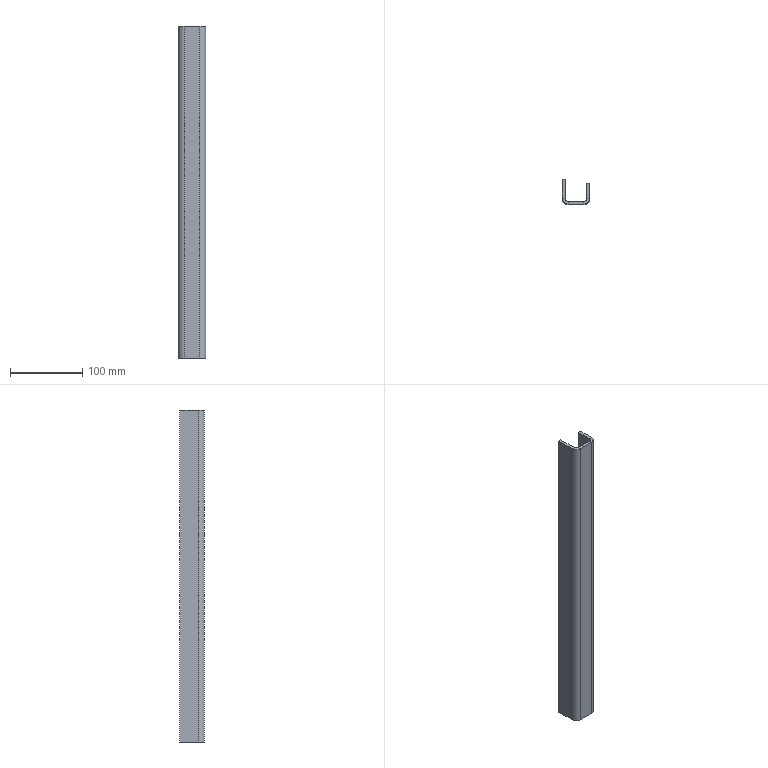Part | STEP file | 07-Reinforcing bent plate 2 | 1 solid | 22 faces | box 38 x 34 x 459 mm | volume 161170 mm3 | plane 18 | cylinder 4 | commonest cylinder face diameters 8 x2 16 x2
STEP:
#1=CARTESIAN_POINT('',(0.,0.,0.));
#2=DIRECTION('',(0.,0.,1.));
#3=DIRECTION('',(1.,0.,0.));
#4=AXIS2_PLACEMENT_3D('',#1,#2,#3);
#5=CARTESIAN_POINT('',(0.,-26.,459.));
#6=VERTEX_POINT('',#5);
#7=CARTESIAN_POINT('',(4.,-26.,459.));
#8=VERTEX_POINT('',#7);
#9=CARTESIAN_POINT('',(0.,-26.,459.));
#10=DIRECTION('',(1.,0.,0.));
#11=VECTOR('',#10,1.);
#12=LINE('',#9,#11);
#13=CARTESIAN_POINT('',(0.,-26.,459.));
#14=DIRECTION('',(0.,0.,1.));
#15=DIRECTION('',(1.,0.,0.));
#16=AXIS2_PLACEMENT_3D('',#13,#14,#15);
#17=PLANE('',#16);
#18=CARTESIAN_POINT('',(0.,0.));
#19=DIRECTION('',(1.,0.));
#20=VECTOR('',#19,1.);
#21=LINE('',#18,#20);
#22=(GEOMETRIC_REPRESENTATION_CONTEXT(2)PARAMETRIC_REPRESENTATION_CONTEXT()REPRESENTATION_CONTEXT('',''));
#23=DEFINITIONAL_REPRESENTATION('',(#21),#22);
#24=PCURVE('',#17,#23);
#25=CARTESIAN_POINT('',(8.,-30.,459.));
#26=DIRECTION('',(0.,0.,1.));
#27=DIRECTION('',(1.,0.,0.));
#28=AXIS2_PLACEMENT_3D('',#25,#26,#27);
#29=PLANE('',#28);
#30=CARTESIAN_POINT('',(-8.,4.));
#31=DIRECTION('',(1.,0.));
#32=VECTOR('',#31,1.);
#33=LINE('',#30,#32);
#34=(GEOMETRIC_REPRESENTATION_CONTEXT(2)PARAMETRIC_REPRESENTATION_CONTEXT()REPRESENTATION_CONTEXT('',''));
#35=DEFINITIONAL_REPRESENTATION('',(#33),#34);
#36=PCURVE('',#29,#35);
#37=SURFACE_CURVE('',#12,(#24,#36),.PCURVE_S1.);
#38=EDGE_CURVE('',#6,#8,#37,.T.);
#39=ORIENTED_EDGE('',*,*,#38,.F.);
#40=CARTESIAN_POINT('',(8.,-34.,459.));
#41=VERTEX_POINT('',#40);
#42=CARTESIAN_POINT('',(8.,-26.,459.));
#43=DIRECTION('',(0.,0.,1.));
#44=DIRECTION('',(-1.,0.,0.));
#45=AXIS2_PLACEMENT_3D('',#42,#43,#44);
#46=CIRCLE('',#45,8.);
#47=CARTESIAN_POINT('',(8.,0.));
#48=DIRECTION('',(-1.,0.));
#49=AXIS2_PLACEMENT_2D('',#47,#48);
#50=CIRCLE('',#49,8.);
#51=(GEOMETRIC_REPRESENTATION_CONTEXT(2)PARAMETRIC_REPRESENTATION_CONTEXT()REPRESENTATION_CONTEXT('',''));
#52=DEFINITIONAL_REPRESENTATION('',(#50),#51);
#53=PCURVE('',#17,#52);
#54=CARTESIAN_POINT('',(8.,-26.,459.));
#55=DIRECTION('',(0.,0.,-1.));
#56=DIRECTION('',(-1.,0.,0.));
#57=AXIS2_PLACEMENT_3D('',#54,#55,#56);
#58=CYLINDRICAL_SURFACE('',#57,8.);
#59=CARTESIAN_POINT('',(6.283,0.));
#60=DIRECTION('',(-1.,0.));
#61=VECTOR('',#60,1.);
#62=LINE('',#59,#61);
#63=(GEOMETRIC_REPRESENTATION_CONTEXT(2)PARAMETRIC_REPRESENTATION_CONTEXT()REPRESENTATION_CONTEXT('',''));
#64=DEFINITIONAL_REPRESENTATION('',(#62),#63);
#65=PCURVE('',#58,#64);
#66=SURFACE_CURVE('',#46,(#53,#65),.PCURVE_S1.);
#67=EDGE_CURVE('',#6,#41,#66,.T.);
#68=ORIENTED_EDGE('',*,*,#67,.T.);
#69=CARTESIAN_POINT('',(8.,-30.,459.));
#70=VERTEX_POINT('',#69);
#71=CARTESIAN_POINT('',(8.,-30.,459.));
#72=DIRECTION('',(0.,-1.,0.));
#73=VECTOR('',#72,1.);
#74=LINE('',#71,#73);
#75=CARTESIAN_POINT('',(8.,-4.));
#76=DIRECTION('',(0.,-1.));
#77=VECTOR('',#76,1.);
#78=LINE('',#75,#77);
#79=(GEOMETRIC_REPRESENTATION_CONTEXT(2)PARAMETRIC_REPRESENTATION_CONTEXT()REPRESENTATION_CONTEXT('',''));
#80=DEFINITIONAL_REPRESENTATION('',(#78),#79);
#81=PCURVE('',#17,#80);
#82=CARTESIAN_POINT('',(34.,-26.,459.));
#83=DIRECTION('',(0.,0.,1.));
#84=DIRECTION('',(1.,0.,0.));
#85=AXIS2_PLACEMENT_3D('',#82,#83,#84);
#86=PLANE('',#85);
#87=CARTESIAN_POINT('',(-26.,-4.));
#88=DIRECTION('',(0.,-1.));
#89=VECTOR('',#88,1.);
#90=LINE('',#87,#89);
#91=(GEOMETRIC_REPRESENTATION_CONTEXT(2)PARAMETRIC_REPRESENTATION_CONTEXT()REPRESENTATION_CONTEXT('',''));
#92=DEFINITIONAL_REPRESENTATION('',(#90),#91);
#93=PCURVE('',#86,#92);
#94=SURFACE_CURVE('',#74,(#81,#93),.PCURVE_S1.);
#95=EDGE_CURVE('',#70,#41,#94,.T.);
#96=ORIENTED_EDGE('',*,*,#95,.F.);
#97=CARTESIAN_POINT('',(8.,-26.,459.));
#98=DIRECTION('',(0.,0.,1.));
#99=DIRECTION('',(1.,0.,0.));
#100=AXIS2_PLACEMENT_3D('',#97,#98,#99);
#101=CIRCLE('',#100,4.);
#102=CARTESIAN_POINT('',(8.,0.));
#103=DIRECTION('',(1.,0.));
#104=AXIS2_PLACEMENT_2D('',#102,#103);
#105=CIRCLE('',#104,4.);
#106=(GEOMETRIC_REPRESENTATION_CONTEXT(2)PARAMETRIC_REPRESENTATION_CONTEXT()REPRESENTATION_CONTEXT('',''));
#107=DEFINITIONAL_REPRESENTATION('',(#105),#106);
#108=PCURVE('',#17,#107);
#109=CARTESIAN_POINT('',(8.,-26.,459.));
#110=DIRECTION('',(0.,0.,-1.));
#111=DIRECTION('',(-1.,0.,0.));
#112=AXIS2_PLACEMENT_3D('',#109,#110,#111);
#113=CYLINDRICAL_SURFACE('',#112,4.);
#114=CARTESIAN_POINT('',(9.425,0.));
#115=DIRECTION('',(-1.,0.));
#116=VECTOR('',#115,1.);
#117=LINE('',#114,#116);
#118=(GEOMETRIC_REPRESENTATION_CONTEXT(2)PARAMETRIC_REPRESENTATION_CONTEXT()REPRESENTATION_CONTEXT('',''));
#119=DEFINITIONAL_REPRESENTATION('',(#117),#118);
#120=PCURVE('',#113,#119);
#121=SURFACE_CURVE('',#101,(#108,#120),.PCURVE_S1.);
#122=EDGE_CURVE('',#8,#70,#121,.T.);
#123=ORIENTED_EDGE('',*,*,#122,.F.);
#124=EDGE_LOOP('',(#39,#68,#96,#123));
#125=FACE_BOUND('',#124,.T.);
#126=ADVANCED_FACE('',(#125),#17,.T.);
#127=CARTESIAN_POINT('',(0.,0.,459.));
#128=VERTEX_POINT('',#127);
#129=CARTESIAN_POINT('',(0.,0.,459.));
#130=DIRECTION('',(0.,-1.,0.));
#131=VECTOR('',#130,1.);
#132=LINE('',#129,#131);
#133=CARTESIAN_POINT('',(-8.,30.));
#134=DIRECTION('',(0.,-1.));
#135=VECTOR('',#134,1.);
#136=LINE('',#133,#135);
#137=(GEOMETRIC_REPRESENTATION_CONTEXT(2)PARAMETRIC_REPRESENTATION_CONTEXT()REPRESENTATION_CONTEXT('',''));
#138=DEFINITIONAL_REPRESENTATION('',(#136),#137);
#139=PCURVE('',#29,#138);
#140=CARTESIAN_POINT('',(0.,0.,459.));
#141=DIRECTION('',(1.,0.,0.));
#142=DIRECTION('',(0.,1.,0.));
#143=AXIS2_PLACEMENT_3D('',#140,#141,#142);
#144=PLANE('',#143);
#145=CARTESIAN_POINT('',(0.,0.));
#146=DIRECTION('',(-1.,0.));
#147=VECTOR('',#146,1.);
#148=LINE('',#145,#147);
#149=(GEOMETRIC_REPRESENTATION_CONTEXT(2)PARAMETRIC_REPRESENTATION_CONTEXT()REPRESENTATION_CONTEXT('',''));
#150=DEFINITIONAL_REPRESENTATION('',(#148),#149);
#151=PCURVE('',#144,#150);
#152=SURFACE_CURVE('',#132,(#139,#151),.PCURVE_S1.);
#153=EDGE_CURVE('',#128,#6,#152,.T.);
#154=ORIENTED_EDGE('',*,*,#153,.T.);
#155=ORIENTED_EDGE('',*,*,#38,.T.);
#156=CARTESIAN_POINT('',(4.,0.,459.));
#157=VERTEX_POINT('',#156);
#158=CARTESIAN_POINT('',(4.,0.,459.));
#159=DIRECTION('',(0.,-1.,0.));
#160=VECTOR('',#159,1.);
#161=LINE('',#158,#160);
#162=CARTESIAN_POINT('',(-4.,30.));
#163=DIRECTION('',(0.,-1.));
#164=VECTOR('',#163,1.);
#165=LINE('',#162,#164);
#166=(GEOMETRIC_REPRESENTATION_CONTEXT(2)PARAMETRIC_REPRESENTATION_CONTEXT()REPRESENTATION_CONTEXT('',''));
#167=DEFINITIONAL_REPRESENTATION('',(#165),#166);
#168=PCURVE('',#29,#167);
#169=CARTESIAN_POINT('',(4.,0.,459.));
#170=DIRECTION('',(1.,0.,0.));
#171=DIRECTION('',(0.,1.,0.));
#172=AXIS2_PLACEMENT_3D('',#169,#170,#171);
#173=PLANE('',#172);
#174=CARTESIAN_POINT('',(0.,0.));
#175=DIRECTION('',(-1.,0.));
#176=VECTOR('',#175,1.);
#177=LINE('',#174,#176);
#178=(GEOMETRIC_REPRESENTATION_CONTEXT(2)PARAMETRIC_REPRESENTATION_CONTEXT()REPRESENTATION_CONTEXT('',''));
#179=DEFINITIONAL_REPRESENTATION('',(#177),#178);
#180=PCURVE('',#173,#179);
#181=SURFACE_CURVE('',#161,(#168,#180),.PCURVE_S1.);
#182=EDGE_CURVE('',#157,#8,#181,.T.);
#183=ORIENTED_EDGE('',*,*,#182,.F.);
#184=CARTESIAN_POINT('',(0.,0.,459.));
#185=DIRECTION('',(1.,0.,0.));
#186=VECTOR('',#185,1.);
#187=LINE('',#184,#186);
#188=CARTESIAN_POINT('',(-8.,30.));
#189=DIRECTION('',(1.,0.));
#190=VECTOR('',#189,1.);
#191=LINE('',#188,#190);
#192=(GEOMETRIC_REPRESENTATION_CONTEXT(2)PARAMETRIC_REPRESENTATION_CONTEXT()REPRESENTATION_CONTEXT('',''));
#193=DEFINITIONAL_REPRESENTATION('',(#191),#192);
#194=PCURVE('',#29,#193);
#195=CARTESIAN_POINT('',(0.,0.,459.));
#196=DIRECTION('',(0.,1.,0.));
#197=DIRECTION('',(-1.,0.,0.));
#198=AXIS2_PLACEMENT_3D('',#195,#196,#197);
#199=PLANE('',#198);
#200=CARTESIAN_POINT('',(0.,0.));
#201=DIRECTION('',(-1.,0.));
#202=VECTOR('',#201,1.);
#203=LINE('',#200,#202);
#204=(GEOMETRIC_REPRESENTATION_CONTEXT(2)PARAMETRIC_REPRESENTATION_CONTEXT()REPRESENTATION_CONTEXT('',''));
#205=DEFINITIONAL_REPRESENTATION('',(#203),#204);
#206=PCURVE('',#199,#205);
#207=SURFACE_CURVE('',#187,(#194,#206),.PCURVE_S1.);
#208=EDGE_CURVE('',#128,#157,#207,.T.);
#209=ORIENTED_EDGE('',*,*,#208,.F.);
#210=EDGE_LOOP('',(#154,#155,#183,#209));
#211=FACE_BOUND('',#210,.T.);
#212=ADVANCED_FACE('',(#211),#29,.T.);
#213=CARTESIAN_POINT('',(8.,-34.,0.));
#214=VERTEX_POINT('',#213);
#215=CARTESIAN_POINT('',(8.,-30.,0.));
#216=VERTEX_POINT('',#215);
#217=CARTESIAN_POINT('',(8.,-34.,0.));
#218=DIRECTION('',(0.,1.,0.));
#219=VECTOR('',#218,1.);
#220=LINE('',#217,#219);
#221=CARTESIAN_POINT('',(8.,-34.,0.));
#222=DIRECTION('',(0.,0.,-1.));
#223=DIRECTION('',(-1.,0.,0.));
#224=AXIS2_PLACEMENT_3D('',#221,#222,#223);
#225=PLANE('',#224);
#226=CARTESIAN_POINT('',(0.,0.));
#227=DIRECTION('',(0.,1.));
#228=VECTOR('',#227,1.);
#229=LINE('',#226,#228);
#230=(GEOMETRIC_REPRESENTATION_CONTEXT(2)PARAMETRIC_REPRESENTATION_CONTEXT()REPRESENTATION_CONTEXT('',''));
#231=DEFINITIONAL_REPRESENTATION('',(#229),#230);
#232=PCURVE('',#225,#231);
#233=CARTESIAN_POINT('',(4.,-26.,0.));
#234=DIRECTION('',(0.,0.,-1.));
#235=DIRECTION('',(-1.,0.,0.));
#236=AXIS2_PLACEMENT_3D('',#233,#234,#235);
#237=PLANE('',#236);
#238=CARTESIAN_POINT('',(-4.,-8.));
#239=DIRECTION('',(0.,1.));
#240=VECTOR('',#239,1.);
#241=LINE('',#238,#240);
#242=(GEOMETRIC_REPRESENTATION_CONTEXT(2)PARAMETRIC_REPRESENTATION_CONTEXT()REPRESENTATION_CONTEXT('',''));
#243=DEFINITIONAL_REPRESENTATION('',(#241),#242);
#244=PCURVE('',#237,#243);
#245=SURFACE_CURVE('',#220,(#232,#244),.PCURVE_S1.);
#246=EDGE_CURVE('',#214,#216,#245,.T.);
#247=ORIENTED_EDGE('',*,*,#246,.F.);
#248=CARTESIAN_POINT('',(0.,-26.,0.));
#249=VERTEX_POINT('',#248);
#250=CARTESIAN_POINT('',(8.,-26.,0.));
#251=DIRECTION('',(0.,0.,1.));
#252=DIRECTION('',(-1.,0.,0.));
#253=AXIS2_PLACEMENT_3D('',#250,#251,#252);
#254=CIRCLE('',#253,8.);
#255=CARTESIAN_POINT('',(8.,8.));
#256=CARTESIAN_POINT('',(8.,-5.856));
#257=CARTESIAN_POINT('',(-4.,1.072));
#258=CARTESIAN_POINT('',(-16.,8.));
#259=CARTESIAN_POINT('',(-4.,14.928));
#260=CARTESIAN_POINT('',(8.,21.856));
#261=CARTESIAN_POINT('',(8.,8.));
#262=(BOUNDED_CURVE()B_SPLINE_CURVE(2,(#255,#256,#257,#258,#259,#260,#261),.UNSPECIFIED.,.T.,.F.)B_SPLINE_CURVE_WITH_KNOTS((1,2,2,2,2,1),(-2.094,0.,2.094,4.189,6.283,8.378),.UNSPECIFIED.)CURVE()GEOMETRIC_REPRESENTATION_ITEM()RATIONAL_B_SPLINE_CURVE((1.,0.5,1.,0.5,1.,0.5,1.))REPRESENTATION_ITEM(''));
#263=(GEOMETRIC_REPRESENTATION_CONTEXT(2)PARAMETRIC_REPRESENTATION_CONTEXT()REPRESENTATION_CONTEXT('',''));
#264=DEFINITIONAL_REPRESENTATION('',(#262),#263);
#265=PCURVE('',#225,#264);
#266=CARTESIAN_POINT('',(6.283,459.));
#267=DIRECTION('',(-1.,0.));
#268=VECTOR('',#267,1.);
#269=LINE('',#266,#268);
#270=(GEOMETRIC_REPRESENTATION_CONTEXT(2)PARAMETRIC_REPRESENTATION_CONTEXT()REPRESENTATION_CONTEXT('',''));
#271=DEFINITIONAL_REPRESENTATION('',(#269),#270);
#272=PCURVE('',#58,#271);
#273=SURFACE_CURVE('',#254,(#265,#272),.PCURVE_S1.);
#274=EDGE_CURVE('',#249,#214,#273,.T.);
#275=ORIENTED_EDGE('',*,*,#274,.F.);
#276=CARTESIAN_POINT('',(4.,-26.,0.));
#277=VERTEX_POINT('',#276);
#278=CARTESIAN_POINT('',(4.,-26.,0.));
#279=DIRECTION('',(-1.,0.,0.));
#280=VECTOR('',#279,1.);
#281=LINE('',#278,#280);
#282=CARTESIAN_POINT('',(4.,8.));
#283=DIRECTION('',(1.,0.));
#284=VECTOR('',#283,1.);
#285=LINE('',#282,#284);
#286=(GEOMETRIC_REPRESENTATION_CONTEXT(2)PARAMETRIC_REPRESENTATION_CONTEXT()REPRESENTATION_CONTEXT('',''));
#287=DEFINITIONAL_REPRESENTATION('',(#285),#286);
#288=PCURVE('',#225,#287);
#289=CARTESIAN_POINT('',(30.,-26.,0.));
#290=DIRECTION('',(0.,0.,1.));
#291=DIRECTION('',(1.,0.,0.));
#292=AXIS2_PLACEMENT_3D('',#289,#290,#291);
#293=PLANE('',#292);
#294=CARTESIAN_POINT('',(-26.,0.));
#295=DIRECTION('',(-1.,0.));
#296=VECTOR('',#295,1.);
#297=LINE('',#294,#296);
#298=(GEOMETRIC_REPRESENTATION_CONTEXT(2)PARAMETRIC_REPRESENTATION_CONTEXT()REPRESENTATION_CONTEXT('',''));
#299=DEFINITIONAL_REPRESENTATION('',(#297),#298);
#300=PCURVE('',#293,#299);
#301=SURFACE_CURVE('',#281,(#288,#300),.PCURVE_S1.);
#302=EDGE_CURVE('',#277,#249,#301,.T.);
#303=ORIENTED_EDGE('',*,*,#302,.F.);
#304=CARTESIAN_POINT('',(8.,-26.,0.));
#305=DIRECTION('',(0.,0.,1.));
#306=DIRECTION('',(1.,0.,0.));
#307=AXIS2_PLACEMENT_3D('',#304,#305,#306);
#308=CIRCLE('',#307,4.);
#309=CARTESIAN_POINT('',(-4.,8.));
#310=CARTESIAN_POINT('',(-4.,14.928));
#311=CARTESIAN_POINT('',(2.,11.464));
#312=CARTESIAN_POINT('',(8.,8.));
#313=CARTESIAN_POINT('',(2.,4.536));
#314=CARTESIAN_POINT('',(-4.,1.072));
#315=CARTESIAN_POINT('',(-4.,8.));
#316=(BOUNDED_CURVE()B_SPLINE_CURVE(2,(#309,#310,#311,#312,#313,#314,#315),.UNSPECIFIED.,.T.,.F.)B_SPLINE_CURVE_WITH_KNOTS((1,2,2,2,2,1),(-2.094,0.,2.094,4.189,6.283,8.378),.UNSPECIFIED.)CURVE()GEOMETRIC_REPRESENTATION_ITEM()RATIONAL_B_SPLINE_CURVE((1.,0.5,1.,0.5,1.,0.5,1.))REPRESENTATION_ITEM(''));
#317=(GEOMETRIC_REPRESENTATION_CONTEXT(2)PARAMETRIC_REPRESENTATION_CONTEXT()REPRESENTATION_CONTEXT('',''));
#318=DEFINITIONAL_REPRESENTATION('',(#316),#317);
#319=PCURVE('',#225,#318);
#320=CARTESIAN_POINT('',(9.425,459.));
#321=DIRECTION('',(-1.,0.));
#322=VECTOR('',#321,1.);
#323=LINE('',#320,#322);
#324=(GEOMETRIC_REPRESENTATION_CONTEXT(2)PARAMETRIC_REPRESENTATION_CONTEXT()REPRESENTATION_CONTEXT('',''));
#325=DEFINITIONAL_REPRESENTATION('',(#323),#324);
#326=PCURVE('',#113,#325);
#327=SURFACE_CURVE('',#308,(#319,#326),.PCURVE_S1.);
#328=EDGE_CURVE('',#277,#216,#327,.T.);
#329=ORIENTED_EDGE('',*,*,#328,.T.);
#330=EDGE_LOOP('',(#247,#275,#303,#329));
#331=FACE_BOUND('',#330,.T.);
#332=ADVANCED_FACE('',(#331),#225,.T.);
#333=CARTESIAN_POINT('',(30.,-34.,0.));
#334=VERTEX_POINT('',#333);
#335=CARTESIAN_POINT('',(0.,-34.,0.));
#336=DIRECTION('',(1.,0.,0.));
#337=VECTOR('',#336,1.);
#338=LINE('',#335,#337);
#339=CARTESIAN_POINT('',(4.,-8.));
#340=DIRECTION('',(-1.,0.));
#341=VECTOR('',#340,1.);
#342=LINE('',#339,#341);
#343=(GEOMETRIC_REPRESENTATION_CONTEXT(2)PARAMETRIC_REPRESENTATION_CONTEXT()REPRESENTATION_CONTEXT('',''));
#344=DEFINITIONAL_REPRESENTATION('',(#342),#343);
#345=PCURVE('',#237,#344);
#346=CARTESIAN_POINT('',(0.,-34.,459.));
#347=DIRECTION('',(0.,1.,0.));
#348=DIRECTION('',(0.,0.,1.));
#349=AXIS2_PLACEMENT_3D('',#346,#347,#348);
#350=PLANE('',#349);
#351=CARTESIAN_POINT('',(-459.,0.));
#352=DIRECTION('',(0.,1.));
#353=VECTOR('',#352,1.);
#354=LINE('',#351,#353);
#355=(GEOMETRIC_REPRESENTATION_CONTEXT(2)PARAMETRIC_REPRESENTATION_CONTEXT()REPRESENTATION_CONTEXT('',''));
#356=DEFINITIONAL_REPRESENTATION('',(#354),#355);
#357=PCURVE('',#350,#356);
#358=SURFACE_CURVE('',#338,(#345,#357),.PCURVE_S1.);
#359=EDGE_CURVE('',#214,#334,#358,.T.);
#360=ORIENTED_EDGE('',*,*,#359,.F.);
#361=ORIENTED_EDGE('',*,*,#246,.T.);
#362=CARTESIAN_POINT('',(30.,-30.,0.));
#363=VERTEX_POINT('',#362);
#364=CARTESIAN_POINT('',(0.,-30.,0.));
#365=DIRECTION('',(1.,0.,0.));
#366=VECTOR('',#365,1.);
#367=LINE('',#364,#366);
#368=CARTESIAN_POINT('',(4.,-4.));
#369=DIRECTION('',(-1.,0.));
#370=VECTOR('',#369,1.);
#371=LINE('',#368,#370);
#372=(GEOMETRIC_REPRESENTATION_CONTEXT(2)PARAMETRIC_REPRESENTATION_CONTEXT()REPRESENTATION_CONTEXT('',''));
#373=DEFINITIONAL_REPRESENTATION('',(#371),#372);
#374=PCURVE('',#237,#373);
#375=CARTESIAN_POINT('',(0.,-30.,459.));
#376=DIRECTION('',(0.,1.,0.));
#377=DIRECTION('',(0.,0.,1.));
#378=AXIS2_PLACEMENT_3D('',#375,#376,#377);
#379=PLANE('',#378);
#380=CARTESIAN_POINT('',(-459.,0.));
#381=DIRECTION('',(0.,1.));
#382=VECTOR('',#381,1.);
#383=LINE('',#380,#382);
#384=(GEOMETRIC_REPRESENTATION_CONTEXT(2)PARAMETRIC_REPRESENTATION_CONTEXT()REPRESENTATION_CONTEXT('',''));
#385=DEFINITIONAL_REPRESENTATION('',(#383),#384);
#386=PCURVE('',#379,#385);
#387=SURFACE_CURVE('',#367,(#374,#386),.PCURVE_S1.);
#388=EDGE_CURVE('',#216,#363,#387,.T.);
#389=ORIENTED_EDGE('',*,*,#388,.T.);
#390=CARTESIAN_POINT('',(30.,-30.,0.));
#391=DIRECTION('',(0.,-1.,0.));
#392=VECTOR('',#391,1.);
#393=LINE('',#390,#392);
#394=CARTESIAN_POINT('',(-26.,-4.));
#395=DIRECTION('',(0.,-1.));
#396=VECTOR('',#395,1.);
#397=LINE('',#394,#396);
#398=(GEOMETRIC_REPRESENTATION_CONTEXT(2)PARAMETRIC_REPRESENTATION_CONTEXT()REPRESENTATION_CONTEXT('',''));
#399=DEFINITIONAL_REPRESENTATION('',(#397),#398);
#400=PCURVE('',#237,#399);
#401=CARTESIAN_POINT('',(38.,-26.,0.));
#402=DIRECTION('',(0.,0.,-1.));
#403=DIRECTION('',(-1.,0.,0.));
#404=AXIS2_PLACEMENT_3D('',#401,#402,#403);
#405=PLANE('',#404);
#406=CARTESIAN_POINT('',(8.,-4.));
#407=DIRECTION('',(0.,-1.));
#408=VECTOR('',#407,1.);
#409=LINE('',#406,#408);
#410=(GEOMETRIC_REPRESENTATION_CONTEXT(2)PARAMETRIC_REPRESENTATION_CONTEXT()REPRESENTATION_CONTEXT('',''));
#411=DEFINITIONAL_REPRESENTATION('',(#409),#410);
#412=PCURVE('',#405,#411);
#413=SURFACE_CURVE('',#393,(#400,#412),.PCURVE_S1.);
#414=EDGE_CURVE('',#363,#334,#413,.T.);
#415=ORIENTED_EDGE('',*,*,#414,.T.);
#416=EDGE_LOOP('',(#360,#361,#389,#415));
#417=FACE_BOUND('',#416,.T.);
#418=ADVANCED_FACE('',(#417),#237,.T.);
#419=CARTESIAN_POINT('',(30.,-34.,459.));
#420=VERTEX_POINT('',#419);
#421=CARTESIAN_POINT('',(30.,-30.,459.));
#422=VERTEX_POINT('',#421);
#423=CARTESIAN_POINT('',(30.,-34.,459.));
#424=DIRECTION('',(0.,1.,0.));
#425=VECTOR('',#424,1.);
#426=LINE('',#423,#425);
#427=CARTESIAN_POINT('',(30.,-34.,459.));
#428=DIRECTION('',(0.,0.,1.));
#429=DIRECTION('',(1.,0.,0.));
#430=AXIS2_PLACEMENT_3D('',#427,#428,#429);
#431=PLANE('',#430);
#432=CARTESIAN_POINT('',(0.,0.));
#433=DIRECTION('',(0.,1.));
#434=VECTOR('',#433,1.);
#435=LINE('',#432,#434);
#436=(GEOMETRIC_REPRESENTATION_CONTEXT(2)PARAMETRIC_REPRESENTATION_CONTEXT()REPRESENTATION_CONTEXT('',''));
#437=DEFINITIONAL_REPRESENTATION('',(#435),#436);
#438=PCURVE('',#431,#437);
#439=CARTESIAN_POINT('',(-4.,-8.));
#440=DIRECTION('',(0.,1.));
#441=VECTOR('',#440,1.);
#442=LINE('',#439,#441);
#443=(GEOMETRIC_REPRESENTATION_CONTEXT(2)PARAMETRIC_REPRESENTATION_CONTEXT()REPRESENTATION_CONTEXT('',''));
#444=DEFINITIONAL_REPRESENTATION('',(#442),#443);
#445=PCURVE('',#86,#444);
#446=SURFACE_CURVE('',#426,(#438,#445),.PCURVE_S1.);
#447=EDGE_CURVE('',#420,#422,#446,.T.);
#448=ORIENTED_EDGE('',*,*,#447,.F.);
#449=CARTESIAN_POINT('',(38.,-26.,459.));
#450=VERTEX_POINT('',#449);
#451=CARTESIAN_POINT('',(30.,-26.,459.));
#452=DIRECTION('',(0.,0.,1.));
#453=DIRECTION('',(-1.,0.,0.));
#454=AXIS2_PLACEMENT_3D('',#451,#452,#453);
#455=CIRCLE('',#454,8.);
#456=CARTESIAN_POINT('',(0.,8.));
#457=DIRECTION('',(-1.,0.));
#458=AXIS2_PLACEMENT_2D('',#456,#457);
#459=CIRCLE('',#458,8.);
#460=(GEOMETRIC_REPRESENTATION_CONTEXT(2)PARAMETRIC_REPRESENTATION_CONTEXT()REPRESENTATION_CONTEXT('',''));
#461=DEFINITIONAL_REPRESENTATION('',(#459),#460);
#462=PCURVE('',#431,#461);
#463=CARTESIAN_POINT('',(30.,-26.,459.));
#464=DIRECTION('',(0.,0.,-1.));
#465=DIRECTION('',(-1.,0.,0.));
#466=AXIS2_PLACEMENT_3D('',#463,#464,#465);
#467=CYLINDRICAL_SURFACE('',#466,8.);
#468=CARTESIAN_POINT('',(6.283,0.));
#469=DIRECTION('',(-1.,0.));
#470=VECTOR('',#469,1.);
#471=LINE('',#468,#470);
#472=(GEOMETRIC_REPRESENTATION_CONTEXT(2)PARAMETRIC_REPRESENTATION_CONTEXT()REPRESENTATION_CONTEXT('',''));
#473=DEFINITIONAL_REPRESENTATION('',(#471),#472);
#474=PCURVE('',#467,#473);
#475=SURFACE_CURVE('',#455,(#462,#474),.PCURVE_S1.);
#476=EDGE_CURVE('',#420,#450,#475,.T.);
#477=ORIENTED_EDGE('',*,*,#476,.T.);
#478=CARTESIAN_POINT('',(34.,-26.,459.));
#479=VERTEX_POINT('',#478);
#480=CARTESIAN_POINT('',(34.,-26.,459.));
#481=DIRECTION('',(1.,0.,0.));
#482=VECTOR('',#481,1.);
#483=LINE('',#480,#482);
#484=CARTESIAN_POINT('',(4.,8.));
#485=DIRECTION('',(1.,0.));
#486=VECTOR('',#485,1.);
#487=LINE('',#484,#486);
#488=(GEOMETRIC_REPRESENTATION_CONTEXT(2)PARAMETRIC_REPRESENTATION_CONTEXT()REPRESENTATION_CONTEXT('',''));
#489=DEFINITIONAL_REPRESENTATION('',(#487),#488);
#490=PCURVE('',#431,#489);
#491=CARTESIAN_POINT('',(30.,-26.,459.));
#492=DIRECTION('',(0.,0.,1.));
#493=DIRECTION('',(1.,0.,0.));
#494=AXIS2_PLACEMENT_3D('',#491,#492,#493);
#495=PLANE('',#494);
#496=CARTESIAN_POINT('',(4.,0.));
#497=DIRECTION('',(1.,0.));
#498=VECTOR('',#497,1.);
#499=LINE('',#496,#498);
#500=(GEOMETRIC_REPRESENTATION_CONTEXT(2)PARAMETRIC_REPRESENTATION_CONTEXT()REPRESENTATION_CONTEXT('',''));
#501=DEFINITIONAL_REPRESENTATION('',(#499),#500);
#502=PCURVE('',#495,#501);
#503=SURFACE_CURVE('',#483,(#490,#502),.PCURVE_S1.);
#504=EDGE_CURVE('',#479,#450,#503,.T.);
#505=ORIENTED_EDGE('',*,*,#504,.F.);
#506=CARTESIAN_POINT('',(30.,-26.,459.));
#507=DIRECTION('',(0.,0.,1.));
#508=DIRECTION('',(1.,0.,0.));
#509=AXIS2_PLACEMENT_3D('',#506,#507,#508);
#510=CIRCLE('',#509,4.);
#511=CARTESIAN_POINT('',(0.,8.));
#512=DIRECTION('',(1.,0.));
#513=AXIS2_PLACEMENT_2D('',#511,#512);
#514=CIRCLE('',#513,4.);
#515=(GEOMETRIC_REPRESENTATION_CONTEXT(2)PARAMETRIC_REPRESENTATION_CONTEXT()REPRESENTATION_CONTEXT('',''));
#516=DEFINITIONAL_REPRESENTATION('',(#514),#515);
#517=PCURVE('',#431,#516);
#518=CARTESIAN_POINT('',(30.,-26.,459.));
#519=DIRECTION('',(0.,0.,-1.));
#520=DIRECTION('',(-1.,0.,0.));
#521=AXIS2_PLACEMENT_3D('',#518,#519,#520);
#522=CYLINDRICAL_SURFACE('',#521,4.);
#523=CARTESIAN_POINT('',(9.425,0.));
#524=DIRECTION('',(-1.,0.));
#525=VECTOR('',#524,1.);
#526=LINE('',#523,#525);
#527=(GEOMETRIC_REPRESENTATION_CONTEXT(2)PARAMETRIC_REPRESENTATION_CONTEXT()REPRESENTATION_CONTEXT('',''));
#528=DEFINITIONAL_REPRESENTATION('',(#526),#527);
#529=PCURVE('',#522,#528);
#530=SURFACE_CURVE('',#510,(#517,#529),.PCURVE_S1.);
#531=EDGE_CURVE('',#422,#479,#530,.T.);
#532=ORIENTED_EDGE('',*,*,#531,.F.);
#533=EDGE_LOOP('',(#448,#477,#505,#532));
#534=FACE_BOUND('',#533,.T.);
#535=ADVANCED_FACE('',(#534),#431,.T.);
#536=CARTESIAN_POINT('',(0.,-34.,459.));
#537=DIRECTION('',(1.,0.,0.));
#538=VECTOR('',#537,1.);
#539=LINE('',#536,#538);
#540=CARTESIAN_POINT('',(-34.,-8.));
#541=DIRECTION('',(1.,0.));
#542=VECTOR('',#541,1.);
#543=LINE('',#540,#542);
#544=(GEOMETRIC_REPRESENTATION_CONTEXT(2)PARAMETRIC_REPRESENTATION_CONTEXT()REPRESENTATION_CONTEXT('',''));
#545=DEFINITIONAL_REPRESENTATION('',(#543),#544);
#546=PCURVE('',#86,#545);
#547=CARTESIAN_POINT('',(0.,0.));
#548=DIRECTION('',(0.,1.));
#549=VECTOR('',#548,1.);
#550=LINE('',#547,#549);
#551=(GEOMETRIC_REPRESENTATION_CONTEXT(2)PARAMETRIC_REPRESENTATION_CONTEXT()REPRESENTATION_CONTEXT('',''));
#552=DEFINITIONAL_REPRESENTATION('',(#550),#551);
#553=PCURVE('',#350,#552);
#554=SURFACE_CURVE('',#539,(#546,#553),.PCURVE_S1.);
#555=EDGE_CURVE('',#41,#420,#554,.T.);
#556=ORIENTED_EDGE('',*,*,#555,.T.);
#557=ORIENTED_EDGE('',*,*,#447,.T.);
#558=CARTESIAN_POINT('',(0.,-30.,459.));
#559=DIRECTION('',(1.,0.,0.));
#560=VECTOR('',#559,1.);
#561=LINE('',#558,#560);
#562=CARTESIAN_POINT('',(-34.,-4.));
#563=DIRECTION('',(1.,0.));
#564=VECTOR('',#563,1.);
#565=LINE('',#562,#564);
#566=(GEOMETRIC_REPRESENTATION_CONTEXT(2)PARAMETRIC_REPRESENTATION_CONTEXT()REPRESENTATION_CONTEXT('',''));
#567=DEFINITIONAL_REPRESENTATION('',(#565),#566);
#568=PCURVE('',#86,#567);
#569=CARTESIAN_POINT('',(0.,0.));
#570=DIRECTION('',(0.,1.));
#571=VECTOR('',#570,1.);
#572=LINE('',#569,#571);
#573=(GEOMETRIC_REPRESENTATION_CONTEXT(2)PARAMETRIC_REPRESENTATION_CONTEXT()REPRESENTATION_CONTEXT('',''));
#574=DEFINITIONAL_REPRESENTATION('',(#572),#573);
#575=PCURVE('',#379,#574);
#576=SURFACE_CURVE('',#561,(#568,#575),.PCURVE_S1.);
#577=EDGE_CURVE('',#70,#422,#576,.T.);
#578=ORIENTED_EDGE('',*,*,#577,.F.);
#579=ORIENTED_EDGE('',*,*,#95,.T.);
#580=EDGE_LOOP('',(#556,#557,#578,#579));
#581=FACE_BOUND('',#580,.T.);
#582=ADVANCED_FACE('',(#581),#86,.T.);
#583=CARTESIAN_POINT('',(38.,-26.,0.));
#584=VERTEX_POINT('',#583);
#585=CARTESIAN_POINT('',(34.,-26.,0.));
#586=VERTEX_POINT('',#585);
#587=CARTESIAN_POINT('',(38.,-26.,0.));
#588=DIRECTION('',(-1.,0.,0.));
#589=VECTOR('',#588,1.);
#590=LINE('',#587,#589);
#591=CARTESIAN_POINT('',(0.,0.));
#592=DIRECTION('',(1.,0.));
#593=VECTOR('',#592,1.);
#594=LINE('',#591,#593);
#595=(GEOMETRIC_REPRESENTATION_CONTEXT(2)PARAMETRIC_REPRESENTATION_CONTEXT()REPRESENTATION_CONTEXT('',''));
#596=DEFINITIONAL_REPRESENTATION('',(#594),#595);
#597=PCURVE('',#405,#596);
#598=CARTESIAN_POINT('',(30.,-30.,0.));
#599=DIRECTION('',(0.,0.,-1.));
#600=DIRECTION('',(-1.,0.,0.));
#601=AXIS2_PLACEMENT_3D('',#598,#599,#600);
#602=PLANE('',#601);
#603=CARTESIAN_POINT('',(-8.,4.));
#604=DIRECTION('',(1.,0.));
#605=VECTOR('',#604,1.);
#606=LINE('',#603,#605);
#607=(GEOMETRIC_REPRESENTATION_CONTEXT(2)PARAMETRIC_REPRESENTATION_CONTEXT()REPRESENTATION_CONTEXT('',''));
#608=DEFINITIONAL_REPRESENTATION('',(#606),#607);
#609=PCURVE('',#602,#608);
#610=SURFACE_CURVE('',#590,(#597,#609),.PCURVE_S1.);
#611=EDGE_CURVE('',#584,#586,#610,.T.);
#612=ORIENTED_EDGE('',*,*,#611,.F.);
#613=CARTESIAN_POINT('',(30.,-26.,0.));
#614=DIRECTION('',(0.,0.,1.));
#615=DIRECTION('',(-1.,0.,0.));
#616=AXIS2_PLACEMENT_3D('',#613,#614,#615);
#617=CIRCLE('',#616,8.);
#618=CARTESIAN_POINT('',(16.,0.));
#619=CARTESIAN_POINT('',(16.,-13.856));
#620=CARTESIAN_POINT('',(4.,-6.928));
#621=CARTESIAN_POINT('',(-8.,0.));
#622=CARTESIAN_POINT('',(4.,6.928));
#623=CARTESIAN_POINT('',(16.,13.856));
#624=CARTESIAN_POINT('',(16.,0.));
#625=(BOUNDED_CURVE()B_SPLINE_CURVE(2,(#618,#619,#620,#621,#622,#623,#624),.UNSPECIFIED.,.T.,.F.)B_SPLINE_CURVE_WITH_KNOTS((1,2,2,2,2,1),(-2.094,0.,2.094,4.189,6.283,8.378),.UNSPECIFIED.)CURVE()GEOMETRIC_REPRESENTATION_ITEM()RATIONAL_B_SPLINE_CURVE((1.,0.5,1.,0.5,1.,0.5,1.))REPRESENTATION_ITEM(''));
#626=(GEOMETRIC_REPRESENTATION_CONTEXT(2)PARAMETRIC_REPRESENTATION_CONTEXT()REPRESENTATION_CONTEXT('',''));
#627=DEFINITIONAL_REPRESENTATION('',(#625),#626);
#628=PCURVE('',#405,#627);
#629=CARTESIAN_POINT('',(6.283,459.));
#630=DIRECTION('',(-1.,0.));
#631=VECTOR('',#630,1.);
#632=LINE('',#629,#631);
#633=(GEOMETRIC_REPRESENTATION_CONTEXT(2)PARAMETRIC_REPRESENTATION_CONTEXT()REPRESENTATION_CONTEXT('',''));
#634=DEFINITIONAL_REPRESENTATION('',(#632),#633);
#635=PCURVE('',#467,#634);
#636=SURFACE_CURVE('',#617,(#628,#635),.PCURVE_S1.);
#637=EDGE_CURVE('',#334,#584,#636,.T.);
#638=ORIENTED_EDGE('',*,*,#637,.F.);
#639=ORIENTED_EDGE('',*,*,#414,.F.);
#640=CARTESIAN_POINT('',(30.,-26.,0.));
#641=DIRECTION('',(0.,0.,1.));
#642=DIRECTION('',(1.,0.,0.));
#643=AXIS2_PLACEMENT_3D('',#640,#641,#642);
#644=CIRCLE('',#643,4.);
#645=CARTESIAN_POINT('',(4.,0.));
#646=CARTESIAN_POINT('',(4.,6.928));
#647=CARTESIAN_POINT('',(10.,3.464));
#648=CARTESIAN_POINT('',(16.,0.));
#649=CARTESIAN_POINT('',(10.,-3.464));
#650=CARTESIAN_POINT('',(4.,-6.928));
#651=CARTESIAN_POINT('',(4.,0.));
#652=(BOUNDED_CURVE()B_SPLINE_CURVE(2,(#645,#646,#647,#648,#649,#650,#651),.UNSPECIFIED.,.T.,.F.)B_SPLINE_CURVE_WITH_KNOTS((1,2,2,2,2,1),(-2.094,0.,2.094,4.189,6.283,8.378),.UNSPECIFIED.)CURVE()GEOMETRIC_REPRESENTATION_ITEM()RATIONAL_B_SPLINE_CURVE((1.,0.5,1.,0.5,1.,0.5,1.))REPRESENTATION_ITEM(''));
#653=(GEOMETRIC_REPRESENTATION_CONTEXT(2)PARAMETRIC_REPRESENTATION_CONTEXT()REPRESENTATION_CONTEXT('',''));
#654=DEFINITIONAL_REPRESENTATION('',(#652),#653);
#655=PCURVE('',#405,#654);
#656=CARTESIAN_POINT('',(9.425,459.));
#657=DIRECTION('',(-1.,0.));
#658=VECTOR('',#657,1.);
#659=LINE('',#656,#658);
#660=(GEOMETRIC_REPRESENTATION_CONTEXT(2)PARAMETRIC_REPRESENTATION_CONTEXT()REPRESENTATION_CONTEXT('',''));
#661=DEFINITIONAL_REPRESENTATION('',(#659),#660);
#662=PCURVE('',#522,#661);
#663=SURFACE_CURVE('',#644,(#655,#662),.PCURVE_S1.);
#664=EDGE_CURVE('',#363,#586,#663,.T.);
#665=ORIENTED_EDGE('',*,*,#664,.T.);
#666=EDGE_LOOP('',(#612,#638,#639,#665));
#667=FACE_BOUND('',#666,.T.);
#668=ADVANCED_FACE('',(#667),#405,.T.);
#669=CARTESIAN_POINT('',(38.,-5.066,0.));
#670=VERTEX_POINT('',#669);
#671=CARTESIAN_POINT('',(38.,-34.,0.));
#672=DIRECTION('',(0.,1.,0.));
#673=VECTOR('',#672,1.);
#674=LINE('',#671,#673);
#675=CARTESIAN_POINT('',(-8.,-4.));
#676=DIRECTION('',(0.,1.));
#677=VECTOR('',#676,1.);
#678=LINE('',#675,#677);
#679=(GEOMETRIC_REPRESENTATION_CONTEXT(2)PARAMETRIC_REPRESENTATION_CONTEXT()REPRESENTATION_CONTEXT('',''));
#680=DEFINITIONAL_REPRESENTATION('',(#678),#679);
#681=PCURVE('',#602,#680);
#682=CARTESIAN_POINT('',(38.,-34.,459.));
#683=DIRECTION('',(-1.,0.,0.));
#684=DIRECTION('',(0.,0.,1.));
#685=AXIS2_PLACEMENT_3D('',#682,#683,#684);
#686=PLANE('',#685);
#687=CARTESIAN_POINT('',(-459.,0.));
#688=DIRECTION('',(0.,1.));
#689=VECTOR('',#688,1.);
#690=LINE('',#687,#689);
#691=(GEOMETRIC_REPRESENTATION_CONTEXT(2)PARAMETRIC_REPRESENTATION_CONTEXT()REPRESENTATION_CONTEXT('',''));
#692=DEFINITIONAL_REPRESENTATION('',(#690),#691);
#693=PCURVE('',#686,#692);
#694=SURFACE_CURVE('',#674,(#681,#693),.PCURVE_S1.);
#695=EDGE_CURVE('',#584,#670,#694,.T.);
#696=ORIENTED_EDGE('',*,*,#695,.F.);
#697=ORIENTED_EDGE('',*,*,#611,.T.);
#698=CARTESIAN_POINT('',(34.,-5.066,0.));
#699=VERTEX_POINT('',#698);
#700=CARTESIAN_POINT('',(34.,-34.,0.));
#701=DIRECTION('',(0.,1.,0.));
#702=VECTOR('',#701,1.);
#703=LINE('',#700,#702);
#704=CARTESIAN_POINT('',(-4.,-4.));
#705=DIRECTION('',(0.,1.));
#706=VECTOR('',#705,1.);
#707=LINE('',#704,#706);
#708=(GEOMETRIC_REPRESENTATION_CONTEXT(2)PARAMETRIC_REPRESENTATION_CONTEXT()REPRESENTATION_CONTEXT('',''));
#709=DEFINITIONAL_REPRESENTATION('',(#707),#708);
#710=PCURVE('',#602,#709);
#711=CARTESIAN_POINT('',(34.,-34.,459.));
#712=DIRECTION('',(-1.,0.,0.));
#713=DIRECTION('',(0.,0.,1.));
#714=AXIS2_PLACEMENT_3D('',#711,#712,#713);
#715=PLANE('',#714);
#716=CARTESIAN_POINT('',(-459.,0.));
#717=DIRECTION('',(0.,1.));
#718=VECTOR('',#717,1.);
#719=LINE('',#716,#718);
#720=(GEOMETRIC_REPRESENTATION_CONTEXT(2)PARAMETRIC_REPRESENTATION_CONTEXT()REPRESENTATION_CONTEXT('',''));
#721=DEFINITIONAL_REPRESENTATION('',(#719),#720);
#722=PCURVE('',#715,#721);
#723=SURFACE_CURVE('',#703,(#710,#722),.PCURVE_S1.);
#724=EDGE_CURVE('',#586,#699,#723,.T.);
#725=ORIENTED_EDGE('',*,*,#724,.T.);
#726=CARTESIAN_POINT('',(34.,-5.066,0.));
#727=DIRECTION('',(1.,0.,0.));
#728=VECTOR('',#727,1.);
#729=LINE('',#726,#728);
#730=CARTESIAN_POINT('',(-4.,24.934));
#731=DIRECTION('',(-1.,0.));
#732=VECTOR('',#731,1.);
#733=LINE('',#730,#732);
#734=(GEOMETRIC_REPRESENTATION_CONTEXT(2)PARAMETRIC_REPRESENTATION_CONTEXT()REPRESENTATION_CONTEXT('',''));
#735=DEFINITIONAL_REPRESENTATION('',(#733),#734);
#736=PCURVE('',#602,#735);
#737=CARTESIAN_POINT('',(34.,-5.066,459.));
#738=DIRECTION('',(0.,1.,0.));
#739=DIRECTION('',(0.,0.,1.));
#740=AXIS2_PLACEMENT_3D('',#737,#738,#739);
#741=PLANE('',#740);
#742=CARTESIAN_POINT('',(-459.,0.));
#743=DIRECTION('',(0.,1.));
#744=VECTOR('',#743,1.);
#745=LINE('',#742,#744);
#746=(GEOMETRIC_REPRESENTATION_CONTEXT(2)PARAMETRIC_REPRESENTATION_CONTEXT()REPRESENTATION_CONTEXT('',''));
#747=DEFINITIONAL_REPRESENTATION('',(#745),#746);
#748=PCURVE('',#741,#747);
#749=SURFACE_CURVE('',#729,(#736,#748),.PCURVE_S1.);
#750=EDGE_CURVE('',#699,#670,#749,.T.);
#751=ORIENTED_EDGE('',*,*,#750,.T.);
#752=EDGE_LOOP('',(#696,#697,#725,#751));
#753=FACE_BOUND('',#752,.T.);
#754=ADVANCED_FACE('',(#753),#602,.T.);
#755=ORIENTED_EDGE('',*,*,#695,.T.);
#756=CARTESIAN_POINT('',(38.,-5.066,459.));
#757=VERTEX_POINT('',#756);
#758=CARTESIAN_POINT('',(38.,-5.066,459.));
#759=DIRECTION('',(0.,0.,-1.));
#760=VECTOR('',#759,1.);
#761=LINE('',#758,#760);
#762=CARTESIAN_POINT('',(0.,28.934));
#763=DIRECTION('',(-1.,0.));
#764=VECTOR('',#763,1.);
#765=LINE('',#762,#764);
#766=(GEOMETRIC_REPRESENTATION_CONTEXT(2)PARAMETRIC_REPRESENTATION_CONTEXT()REPRESENTATION_CONTEXT('',''));
#767=DEFINITIONAL_REPRESENTATION('',(#765),#766);
#768=PCURVE('',#686,#767);
#769=CARTESIAN_POINT('',(0.,4.));
#770=DIRECTION('',(-1.,0.));
#771=VECTOR('',#770,1.);
#772=LINE('',#769,#771);
#773=(GEOMETRIC_REPRESENTATION_CONTEXT(2)PARAMETRIC_REPRESENTATION_CONTEXT()REPRESENTATION_CONTEXT('',''));
#774=DEFINITIONAL_REPRESENTATION('',(#772),#773);
#775=PCURVE('',#741,#774);
#776=SURFACE_CURVE('',#761,(#768,#775),.PCURVE_S1.);
#777=EDGE_CURVE('',#757,#670,#776,.T.);
#778=ORIENTED_EDGE('',*,*,#777,.F.);
#779=CARTESIAN_POINT('',(38.,-34.,459.));
#780=DIRECTION('',(0.,1.,0.));
#781=VECTOR('',#780,1.);
#782=LINE('',#779,#781);
#783=CARTESIAN_POINT('',(0.,0.));
#784=DIRECTION('',(0.,1.));
#785=VECTOR('',#784,1.);
#786=LINE('',#783,#785);
#787=(GEOMETRIC_REPRESENTATION_CONTEXT(2)PARAMETRIC_REPRESENTATION_CONTEXT()REPRESENTATION_CONTEXT('',''));
#788=DEFINITIONAL_REPRESENTATION('',(#786),#787);
#789=PCURVE('',#686,#788);
#790=CARTESIAN_POINT('',(8.,-8.));
#791=DIRECTION('',(0.,1.));
#792=VECTOR('',#791,1.);
#793=LINE('',#790,#792);
#794=(GEOMETRIC_REPRESENTATION_CONTEXT(2)PARAMETRIC_REPRESENTATION_CONTEXT()REPRESENTATION_CONTEXT('',''));
#795=DEFINITIONAL_REPRESENTATION('',(#793),#794);
#796=PCURVE('',#495,#795);
#797=SURFACE_CURVE('',#782,(#789,#796),.PCURVE_S1.);
#798=EDGE_CURVE('',#450,#757,#797,.T.);
#799=ORIENTED_EDGE('',*,*,#798,.F.);
#800=CARTESIAN_POINT('',(38.,-26.,459.));
#801=DIRECTION('',(0.,0.,-1.));
#802=VECTOR('',#801,1.);
#803=LINE('',#800,#802);
#804=CARTESIAN_POINT('',(0.,8.));
#805=DIRECTION('',(-1.,0.));
#806=VECTOR('',#805,1.);
#807=LINE('',#804,#806);
#808=(GEOMETRIC_REPRESENTATION_CONTEXT(2)PARAMETRIC_REPRESENTATION_CONTEXT()REPRESENTATION_CONTEXT('',''));
#809=DEFINITIONAL_REPRESENTATION('',(#807),#808);
#810=PCURVE('',#686,#809);
#811=CARTESIAN_POINT('',(3.142,0.));
#812=DIRECTION('',(0.,1.));
#813=VECTOR('',#812,1.);
#814=LINE('',#811,#813);
#815=(GEOMETRIC_REPRESENTATION_CONTEXT(2)PARAMETRIC_REPRESENTATION_CONTEXT()REPRESENTATION_CONTEXT('',''));
#816=DEFINITIONAL_REPRESENTATION('',(#814),#815);
#817=PCURVE('',#467,#816);
#818=SURFACE_CURVE('',#803,(#810,#817),.PCURVE_S1.);
#819=EDGE_CURVE('',#450,#584,#818,.T.);
#820=ORIENTED_EDGE('',*,*,#819,.T.);
#821=EDGE_LOOP('',(#755,#778,#799,#820));
#822=FACE_BOUND('',#821,.T.);
#823=ADVANCED_FACE('',(#822),#686,.F.);
#824=ORIENTED_EDGE('',*,*,#750,.F.);
#825=CARTESIAN_POINT('',(34.,-5.066,459.));
#826=VERTEX_POINT('',#825);
#827=CARTESIAN_POINT('',(34.,-5.066,459.));
#828=DIRECTION('',(0.,0.,-1.));
#829=VECTOR('',#828,1.);
#830=LINE('',#827,#829);
#831=CARTESIAN_POINT('',(0.,0.));
#832=DIRECTION('',(-1.,0.));
#833=VECTOR('',#832,1.);
#834=LINE('',#831,#833);
#835=(GEOMETRIC_REPRESENTATION_CONTEXT(2)PARAMETRIC_REPRESENTATION_CONTEXT()REPRESENTATION_CONTEXT('',''));
#836=DEFINITIONAL_REPRESENTATION('',(#834),#835);
#837=PCURVE('',#741,#836);
#838=CARTESIAN_POINT('',(0.,28.934));
#839=DIRECTION('',(-1.,0.));
#840=VECTOR('',#839,1.);
#841=LINE('',#838,#840);
#842=(GEOMETRIC_REPRESENTATION_CONTEXT(2)PARAMETRIC_REPRESENTATION_CONTEXT()REPRESENTATION_CONTEXT('',''));
#843=DEFINITIONAL_REPRESENTATION('',(#841),#842);
#844=PCURVE('',#715,#843);
#845=SURFACE_CURVE('',#830,(#837,#844),.PCURVE_S1.);
#846=EDGE_CURVE('',#826,#699,#845,.T.);
#847=ORIENTED_EDGE('',*,*,#846,.F.);
#848=CARTESIAN_POINT('',(34.,-5.066,459.));
#849=DIRECTION('',(1.,0.,0.));
#850=VECTOR('',#849,1.);
#851=LINE('',#848,#850);
#852=CARTESIAN_POINT('',(0.,0.));
#853=DIRECTION('',(0.,1.));
#854=VECTOR('',#853,1.);
#855=LINE('',#852,#854);
#856=(GEOMETRIC_REPRESENTATION_CONTEXT(2)PARAMETRIC_REPRESENTATION_CONTEXT()REPRESENTATION_CONTEXT('',''));
#857=DEFINITIONAL_REPRESENTATION('',(#855),#856);
#858=PCURVE('',#741,#857);
#859=CARTESIAN_POINT('',(4.,20.934));
#860=DIRECTION('',(1.,0.));
#861=VECTOR('',#860,1.);
#862=LINE('',#859,#861);
#863=(GEOMETRIC_REPRESENTATION_CONTEXT(2)PARAMETRIC_REPRESENTATION_CONTEXT()REPRESENTATION_CONTEXT('',''));
#864=DEFINITIONAL_REPRESENTATION('',(#862),#863);
#865=PCURVE('',#495,#864);
#866=SURFACE_CURVE('',#851,(#858,#865),.PCURVE_S1.);
#867=EDGE_CURVE('',#826,#757,#866,.T.);
#868=ORIENTED_EDGE('',*,*,#867,.T.);
#869=ORIENTED_EDGE('',*,*,#777,.T.);
#870=EDGE_LOOP('',(#824,#847,#868,#869));
#871=FACE_BOUND('',#870,.T.);
#872=ADVANCED_FACE('',(#871),#741,.T.);
#873=ORIENTED_EDGE('',*,*,#724,.F.);
#874=CARTESIAN_POINT('',(34.,-26.,459.));
#875=DIRECTION('',(0.,0.,-1.));
#876=VECTOR('',#875,1.);
#877=LINE('',#874,#876);
#878=CARTESIAN_POINT('',(0.,8.));
#879=DIRECTION('',(-1.,0.));
#880=VECTOR('',#879,1.);
#881=LINE('',#878,#880);
#882=(GEOMETRIC_REPRESENTATION_CONTEXT(2)PARAMETRIC_REPRESENTATION_CONTEXT()REPRESENTATION_CONTEXT('',''));
#883=DEFINITIONAL_REPRESENTATION('',(#881),#882);
#884=PCURVE('',#715,#883);
#885=CARTESIAN_POINT('',(3.142,0.));
#886=DIRECTION('',(0.,1.));
#887=VECTOR('',#886,1.);
#888=LINE('',#885,#887);
#889=(GEOMETRIC_REPRESENTATION_CONTEXT(2)PARAMETRIC_REPRESENTATION_CONTEXT()REPRESENTATION_CONTEXT('',''));
#890=DEFINITIONAL_REPRESENTATION('',(#888),#889);
#891=PCURVE('',#522,#890);
#892=SURFACE_CURVE('',#877,(#884,#891),.PCURVE_S1.);
#893=EDGE_CURVE('',#479,#586,#892,.T.);
#894=ORIENTED_EDGE('',*,*,#893,.F.);
#895=CARTESIAN_POINT('',(34.,-34.,459.));
#896=DIRECTION('',(0.,1.,0.));
#897=VECTOR('',#896,1.);
#898=LINE('',#895,#897);
#899=CARTESIAN_POINT('',(0.,0.));
#900=DIRECTION('',(0.,1.));
#901=VECTOR('',#900,1.);
#902=LINE('',#899,#901);
#903=(GEOMETRIC_REPRESENTATION_CONTEXT(2)PARAMETRIC_REPRESENTATION_CONTEXT()REPRESENTATION_CONTEXT('',''));
#904=DEFINITIONAL_REPRESENTATION('',(#902),#903);
#905=PCURVE('',#715,#904);
#906=CARTESIAN_POINT('',(4.,-8.));
#907=DIRECTION('',(0.,1.));
#908=VECTOR('',#907,1.);
#909=LINE('',#906,#908);
#910=(GEOMETRIC_REPRESENTATION_CONTEXT(2)PARAMETRIC_REPRESENTATION_CONTEXT()REPRESENTATION_CONTEXT('',''));
#911=DEFINITIONAL_REPRESENTATION('',(#909),#910);
#912=PCURVE('',#495,#911);
#913=SURFACE_CURVE('',#898,(#905,#912),.PCURVE_S1.);
#914=EDGE_CURVE('',#479,#826,#913,.T.);
#915=ORIENTED_EDGE('',*,*,#914,.T.);
#916=ORIENTED_EDGE('',*,*,#846,.T.);
#917=EDGE_LOOP('',(#873,#894,#915,#916));
#918=FACE_BOUND('',#917,.T.);
#919=ADVANCED_FACE('',(#918),#715,.T.);
#920=ORIENTED_EDGE('',*,*,#893,.F.);
#921=ORIENTED_EDGE('',*,*,#531,.F.);
#922=CARTESIAN_POINT('',(30.,-30.,459.));
#923=DIRECTION('',(0.,0.,-1.));
#924=VECTOR('',#923,1.);
#925=LINE('',#922,#924);
#926=CARTESIAN_POINT('',(4.712,0.));
#927=DIRECTION('',(0.,1.));
#928=VECTOR('',#927,1.);
#929=LINE('',#926,#928);
#930=(GEOMETRIC_REPRESENTATION_CONTEXT(2)PARAMETRIC_REPRESENTATION_CONTEXT()REPRESENTATION_CONTEXT('',''));
#931=DEFINITIONAL_REPRESENTATION('',(#929),#930);
#932=PCURVE('',#522,#931);
#933=CARTESIAN_POINT('',(0.,30.));
#934=DIRECTION('',(-1.,0.));
#935=VECTOR('',#934,1.);
#936=LINE('',#933,#935);
#937=(GEOMETRIC_REPRESENTATION_CONTEXT(2)PARAMETRIC_REPRESENTATION_CONTEXT()REPRESENTATION_CONTEXT('',''));
#938=DEFINITIONAL_REPRESENTATION('',(#936),#937);
#939=PCURVE('',#379,#938);
#940=SURFACE_CURVE('',#925,(#932,#939),.PCURVE_S1.);
#941=EDGE_CURVE('',#422,#363,#940,.T.);
#942=ORIENTED_EDGE('',*,*,#941,.T.);
#943=ORIENTED_EDGE('',*,*,#664,.T.);
#944=EDGE_LOOP('',(#920,#921,#942,#943));
#945=FACE_BOUND('',#944,.F.);
#946=ADVANCED_FACE('',(#945),#522,.F.);
#947=ORIENTED_EDGE('',*,*,#388,.F.);
#948=CARTESIAN_POINT('',(8.,-30.,459.));
#949=DIRECTION('',(0.,0.,-1.));
#950=VECTOR('',#949,1.);
#951=LINE('',#948,#950);
#952=CARTESIAN_POINT('',(0.,8.));
#953=DIRECTION('',(-1.,0.));
#954=VECTOR('',#953,1.);
#955=LINE('',#952,#954);
#956=(GEOMETRIC_REPRESENTATION_CONTEXT(2)PARAMETRIC_REPRESENTATION_CONTEXT()REPRESENTATION_CONTEXT('',''));
#957=DEFINITIONAL_REPRESENTATION('',(#955),#956);
#958=PCURVE('',#379,#957);
#959=CARTESIAN_POINT('',(4.712,0.));
#960=DIRECTION('',(0.,1.));
#961=VECTOR('',#960,1.);
#962=LINE('',#959,#961);
#963=(GEOMETRIC_REPRESENTATION_CONTEXT(2)PARAMETRIC_REPRESENTATION_CONTEXT()REPRESENTATION_CONTEXT('',''));
#964=DEFINITIONAL_REPRESENTATION('',(#962),#963);
#965=PCURVE('',#113,#964);
#966=SURFACE_CURVE('',#951,(#958,#965),.PCURVE_S1.);
#967=EDGE_CURVE('',#70,#216,#966,.T.);
#968=ORIENTED_EDGE('',*,*,#967,.F.);
#969=ORIENTED_EDGE('',*,*,#577,.T.);
#970=ORIENTED_EDGE('',*,*,#941,.T.);
#971=EDGE_LOOP('',(#947,#968,#969,#970));
#972=FACE_BOUND('',#971,.T.);
#973=ADVANCED_FACE('',(#972),#379,.T.);
#974=ORIENTED_EDGE('',*,*,#967,.F.);
#975=ORIENTED_EDGE('',*,*,#122,.F.);
#976=CARTESIAN_POINT('',(4.,-26.,459.));
#977=DIRECTION('',(0.,0.,-1.));
#978=VECTOR('',#977,1.);
#979=LINE('',#976,#978);
#980=CARTESIAN_POINT('',(6.283,0.));
#981=DIRECTION('',(0.,1.));
#982=VECTOR('',#981,1.);
#983=LINE('',#980,#982);
#984=(GEOMETRIC_REPRESENTATION_CONTEXT(2)PARAMETRIC_REPRESENTATION_CONTEXT()REPRESENTATION_CONTEXT('',''));
#985=DEFINITIONAL_REPRESENTATION('',(#983),#984);
#986=PCURVE('',#113,#985);
#987=CARTESIAN_POINT('',(-26.,0.));
#988=DIRECTION('',(0.,-1.));
#989=VECTOR('',#988,1.);
#990=LINE('',#987,#989);
#991=(GEOMETRIC_REPRESENTATION_CONTEXT(2)PARAMETRIC_REPRESENTATION_CONTEXT()REPRESENTATION_CONTEXT('',''));
#992=DEFINITIONAL_REPRESENTATION('',(#990),#991);
#993=PCURVE('',#173,#992);
#994=SURFACE_CURVE('',#979,(#986,#993),.PCURVE_S1.);
#995=EDGE_CURVE('',#8,#277,#994,.T.);
#996=ORIENTED_EDGE('',*,*,#995,.T.);
#997=ORIENTED_EDGE('',*,*,#328,.T.);
#998=EDGE_LOOP('',(#974,#975,#996,#997));
#999=FACE_BOUND('',#998,.F.);
#1000=ADVANCED_FACE('',(#999),#113,.F.);
#1001=CARTESIAN_POINT('',(4.,0.,0.));
#1002=VERTEX_POINT('',#1001);
#1003=CARTESIAN_POINT('',(4.,0.,0.));
#1004=DIRECTION('',(0.,-1.,0.));
#1005=VECTOR('',#1004,1.);
#1006=LINE('',#1003,#1005);
#1007=CARTESIAN_POINT('',(0.,-459.));
#1008=DIRECTION('',(-1.,0.));
#1009=VECTOR('',#1008,1.);
#1010=LINE('',#1007,#1009);
#1011=(GEOMETRIC_REPRESENTATION_CONTEXT(2)PARAMETRIC_REPRESENTATION_CONTEXT()REPRESENTATION_CONTEXT('',''));
#1012=DEFINITIONAL_REPRESENTATION('',(#1010),#1011);
#1013=PCURVE('',#173,#1012);
#1014=CARTESIAN_POINT('',(-26.,26.));
#1015=DIRECTION('',(0.,-1.));
#1016=VECTOR('',#1015,1.);
#1017=LINE('',#1014,#1016);
#1018=(GEOMETRIC_REPRESENTATION_CONTEXT(2)PARAMETRIC_REPRESENTATION_CONTEXT()REPRESENTATION_CONTEXT('',''));
#1019=DEFINITIONAL_REPRESENTATION('',(#1017),#1018);
#1020=PCURVE('',#293,#1019);
#1021=SURFACE_CURVE('',#1006,(#1013,#1020),.PCURVE_S1.);
#1022=EDGE_CURVE('',#1002,#277,#1021,.T.);
#1023=ORIENTED_EDGE('',*,*,#1022,.F.);
#1024=CARTESIAN_POINT('',(4.,0.,459.));
#1025=DIRECTION('',(0.,0.,-1.));
#1026=VECTOR('',#1025,1.);
#1027=LINE('',#1024,#1026);
#1028=CARTESIAN_POINT('',(0.,0.));
#1029=DIRECTION('',(0.,-1.));
#1030=VECTOR('',#1029,1.);
#1031=LINE('',#1028,#1030);
#1032=(GEOMETRIC_REPRESENTATION_CONTEXT(2)PARAMETRIC_REPRESENTATION_CONTEXT()REPRESENTATION_CONTEXT('',''));
#1033=DEFINITIONAL_REPRESENTATION('',(#1031),#1032);
#1034=PCURVE('',#173,#1033);
#1035=CARTESIAN_POINT('',(-4.,0.));
#1036=DIRECTION('',(0.,-1.));
#1037=VECTOR('',#1036,1.);
#1038=LINE('',#1035,#1037);
#1039=(GEOMETRIC_REPRESENTATION_CONTEXT(2)PARAMETRIC_REPRESENTATION_CONTEXT()REPRESENTATION_CONTEXT('',''));
#1040=DEFINITIONAL_REPRESENTATION('',(#1038),#1039);
#1041=PCURVE('',#199,#1040);
#1042=SURFACE_CURVE('',#1027,(#1034,#1041),.PCURVE_S1.);
#1043=EDGE_CURVE('',#157,#1002,#1042,.T.);
#1044=ORIENTED_EDGE('',*,*,#1043,.F.);
#1045=ORIENTED_EDGE('',*,*,#182,.T.);
#1046=ORIENTED_EDGE('',*,*,#995,.T.);
#1047=EDGE_LOOP('',(#1023,#1044,#1045,#1046));
#1048=FACE_BOUND('',#1047,.T.);
#1049=ADVANCED_FACE('',(#1048),#173,.T.);
#1050=CARTESIAN_POINT('',(0.,0.,0.));
#1051=VERTEX_POINT('',#1050);
#1052=CARTESIAN_POINT('',(0.,0.,0.));
#1053=DIRECTION('',(1.,0.,0.));
#1054=VECTOR('',#1053,1.);
#1055=LINE('',#1052,#1054);
#1056=CARTESIAN_POINT('',(0.,-459.));
#1057=DIRECTION('',(-1.,0.));
#1058=VECTOR('',#1057,1.);
#1059=LINE('',#1056,#1058);
#1060=(GEOMETRIC_REPRESENTATION_CONTEXT(2)PARAMETRIC_REPRESENTATION_CONTEXT()REPRESENTATION_CONTEXT('',''));
#1061=DEFINITIONAL_REPRESENTATION('',(#1059),#1060);
#1062=PCURVE('',#199,#1061);
#1063=CARTESIAN_POINT('',(-30.,26.));
#1064=DIRECTION('',(1.,0.));
#1065=VECTOR('',#1064,1.);
#1066=LINE('',#1063,#1065);
#1067=(GEOMETRIC_REPRESENTATION_CONTEXT(2)PARAMETRIC_REPRESENTATION_CONTEXT()REPRESENTATION_CONTEXT('',''));
#1068=DEFINITIONAL_REPRESENTATION('',(#1066),#1067);
#1069=PCURVE('',#293,#1068);
#1070=SURFACE_CURVE('',#1055,(#1062,#1069),.PCURVE_S1.);
#1071=EDGE_CURVE('',#1051,#1002,#1070,.T.);
#1072=ORIENTED_EDGE('',*,*,#1071,.F.);
#1073=CARTESIAN_POINT('',(0.,0.,459.));
#1074=DIRECTION('',(0.,0.,-1.));
#1075=VECTOR('',#1074,1.);
#1076=LINE('',#1073,#1075);
#1077=CARTESIAN_POINT('',(0.,0.));
#1078=DIRECTION('',(0.,-1.));
#1079=VECTOR('',#1078,1.);
#1080=LINE('',#1077,#1079);
#1081=(GEOMETRIC_REPRESENTATION_CONTEXT(2)PARAMETRIC_REPRESENTATION_CONTEXT()REPRESENTATION_CONTEXT('',''));
#1082=DEFINITIONAL_REPRESENTATION('',(#1080),#1081);
#1083=PCURVE('',#199,#1082);
#1084=CARTESIAN_POINT('',(0.,0.));
#1085=DIRECTION('',(0.,-1.));
#1086=VECTOR('',#1085,1.);
#1087=LINE('',#1084,#1086);
#1088=(GEOMETRIC_REPRESENTATION_CONTEXT(2)PARAMETRIC_REPRESENTATION_CONTEXT()REPRESENTATION_CONTEXT('',''));
#1089=DEFINITIONAL_REPRESENTATION('',(#1087),#1088);
#1090=PCURVE('',#144,#1089);
#1091=SURFACE_CURVE('',#1076,(#1083,#1090),.PCURVE_S1.);
#1092=EDGE_CURVE('',#128,#1051,#1091,.T.);
#1093=ORIENTED_EDGE('',*,*,#1092,.F.);
#1094=ORIENTED_EDGE('',*,*,#208,.T.);
#1095=ORIENTED_EDGE('',*,*,#1043,.T.);
#1096=EDGE_LOOP('',(#1072,#1093,#1094,#1095));
#1097=FACE_BOUND('',#1096,.T.);
#1098=ADVANCED_FACE('',(#1097),#199,.T.);
#1099=CARTESIAN_POINT('',(0.,0.,0.));
#1100=DIRECTION('',(0.,-1.,0.));
#1101=VECTOR('',#1100,1.);
#1102=LINE('',#1099,#1101);
#1103=CARTESIAN_POINT('',(0.,-459.));
#1104=DIRECTION('',(-1.,0.));
#1105=VECTOR('',#1104,1.);
#1106=LINE('',#1103,#1105);
#1107=(GEOMETRIC_REPRESENTATION_CONTEXT(2)PARAMETRIC_REPRESENTATION_CONTEXT()REPRESENTATION_CONTEXT('',''));
#1108=DEFINITIONAL_REPRESENTATION('',(#1106),#1107);
#1109=PCURVE('',#144,#1108);
#1110=CARTESIAN_POINT('',(-30.,26.));
#1111=DIRECTION('',(0.,-1.));
#1112=VECTOR('',#1111,1.);
#1113=LINE('',#1110,#1112);
#1114=(GEOMETRIC_REPRESENTATION_CONTEXT(2)PARAMETRIC_REPRESENTATION_CONTEXT()REPRESENTATION_CONTEXT('',''));
#1115=DEFINITIONAL_REPRESENTATION('',(#1113),#1114);
#1116=PCURVE('',#293,#1115);
#1117=SURFACE_CURVE('',#1102,(#1109,#1116),.PCURVE_S1.);
#1118=EDGE_CURVE('',#1051,#249,#1117,.T.);
#1119=ORIENTED_EDGE('',*,*,#1118,.T.);
#1120=CARTESIAN_POINT('',(0.,-26.,459.));
#1121=DIRECTION('',(0.,0.,-1.));
#1122=VECTOR('',#1121,1.);
#1123=LINE('',#1120,#1122);
#1124=CARTESIAN_POINT('',(-26.,0.));
#1125=DIRECTION('',(0.,-1.));
#1126=VECTOR('',#1125,1.);
#1127=LINE('',#1124,#1126);
#1128=(GEOMETRIC_REPRESENTATION_CONTEXT(2)PARAMETRIC_REPRESENTATION_CONTEXT()REPRESENTATION_CONTEXT('',''));
#1129=DEFINITIONAL_REPRESENTATION('',(#1127),#1128);
#1130=PCURVE('',#144,#1129);
#1131=CARTESIAN_POINT('',(6.283,0.));
#1132=DIRECTION('',(0.,1.));
#1133=VECTOR('',#1132,1.);
#1134=LINE('',#1131,#1133);
#1135=(GEOMETRIC_REPRESENTATION_CONTEXT(2)PARAMETRIC_REPRESENTATION_CONTEXT()REPRESENTATION_CONTEXT('',''));
#1136=DEFINITIONAL_REPRESENTATION('',(#1134),#1135);
#1137=PCURVE('',#58,#1136);
#1138=SURFACE_CURVE('',#1123,(#1130,#1137),.PCURVE_S1.);
#1139=EDGE_CURVE('',#6,#249,#1138,.T.);
#1140=ORIENTED_EDGE('',*,*,#1139,.F.);
#1141=ORIENTED_EDGE('',*,*,#153,.F.);
#1142=ORIENTED_EDGE('',*,*,#1092,.T.);
#1143=EDGE_LOOP('',(#1119,#1140,#1141,#1142));
#1144=FACE_BOUND('',#1143,.T.);
#1145=ADVANCED_FACE('',(#1144),#144,.F.);
#1146=ORIENTED_EDGE('',*,*,#274,.T.);
#1147=CARTESIAN_POINT('',(8.,-34.,459.));
#1148=DIRECTION('',(0.,0.,-1.));
#1149=VECTOR('',#1148,1.);
#1150=LINE('',#1147,#1149);
#1151=CARTESIAN_POINT('',(4.712,0.));
#1152=DIRECTION('',(0.,1.));
#1153=VECTOR('',#1152,1.);
#1154=LINE('',#1151,#1153);
#1155=(GEOMETRIC_REPRESENTATION_CONTEXT(2)PARAMETRIC_REPRESENTATION_CONTEXT()REPRESENTATION_CONTEXT('',''));
#1156=DEFINITIONAL_REPRESENTATION('',(#1154),#1155);
#1157=PCURVE('',#58,#1156);
#1158=CARTESIAN_POINT('',(0.,8.));
#1159=DIRECTION('',(-1.,0.));
#1160=VECTOR('',#1159,1.);
#1161=LINE('',#1158,#1160);
#1162=(GEOMETRIC_REPRESENTATION_CONTEXT(2)PARAMETRIC_REPRESENTATION_CONTEXT()REPRESENTATION_CONTEXT('',''));
#1163=DEFINITIONAL_REPRESENTATION('',(#1161),#1162);
#1164=PCURVE('',#350,#1163);
#1165=SURFACE_CURVE('',#1150,(#1157,#1164),.PCURVE_S1.);
#1166=EDGE_CURVE('',#41,#214,#1165,.T.);
#1167=ORIENTED_EDGE('',*,*,#1166,.F.);
#1168=ORIENTED_EDGE('',*,*,#67,.F.);
#1169=ORIENTED_EDGE('',*,*,#1139,.T.);
#1170=EDGE_LOOP('',(#1146,#1167,#1168,#1169));
#1171=FACE_BOUND('',#1170,.T.);
#1172=ADVANCED_FACE('',(#1171),#58,.T.);
#1173=ORIENTED_EDGE('',*,*,#359,.T.);
#1174=CARTESIAN_POINT('',(30.,-34.,459.));
#1175=DIRECTION('',(0.,0.,-1.));
#1176=VECTOR('',#1175,1.);
#1177=LINE('',#1174,#1176);
#1178=CARTESIAN_POINT('',(0.,30.));
#1179=DIRECTION('',(-1.,0.));
#1180=VECTOR('',#1179,1.);
#1181=LINE('',#1178,#1180);
#1182=(GEOMETRIC_REPRESENTATION_CONTEXT(2)PARAMETRIC_REPRESENTATION_CONTEXT()REPRESENTATION_CONTEXT('',''));
#1183=DEFINITIONAL_REPRESENTATION('',(#1181),#1182);
#1184=PCURVE('',#350,#1183);
#1185=CARTESIAN_POINT('',(4.712,0.));
#1186=DIRECTION('',(0.,1.));
#1187=VECTOR('',#1186,1.);
#1188=LINE('',#1185,#1187);
#1189=(GEOMETRIC_REPRESENTATION_CONTEXT(2)PARAMETRIC_REPRESENTATION_CONTEXT()REPRESENTATION_CONTEXT('',''));
#1190=DEFINITIONAL_REPRESENTATION('',(#1188),#1189);
#1191=PCURVE('',#467,#1190);
#1192=SURFACE_CURVE('',#1177,(#1184,#1191),.PCURVE_S1.);
#1193=EDGE_CURVE('',#420,#334,#1192,.T.);
#1194=ORIENTED_EDGE('',*,*,#1193,.F.);
#1195=ORIENTED_EDGE('',*,*,#555,.F.);
#1196=ORIENTED_EDGE('',*,*,#1166,.T.);
#1197=EDGE_LOOP('',(#1173,#1194,#1195,#1196));
#1198=FACE_BOUND('',#1197,.T.);
#1199=ADVANCED_FACE('',(#1198),#350,.F.);
#1200=ORIENTED_EDGE('',*,*,#637,.T.);
#1201=ORIENTED_EDGE('',*,*,#819,.F.);
#1202=ORIENTED_EDGE('',*,*,#476,.F.);
#1203=ORIENTED_EDGE('',*,*,#1193,.T.);
#1204=EDGE_LOOP('',(#1200,#1201,#1202,#1203));
#1205=FACE_BOUND('',#1204,.T.);
#1206=ADVANCED_FACE('',(#1205),#467,.T.);
#1207=ORIENTED_EDGE('',*,*,#798,.T.);
#1208=ORIENTED_EDGE('',*,*,#867,.F.);
#1209=ORIENTED_EDGE('',*,*,#914,.F.);
#1210=ORIENTED_EDGE('',*,*,#504,.T.);
#1211=EDGE_LOOP('',(#1207,#1208,#1209,#1210));
#1212=FACE_BOUND('',#1211,.T.);
#1213=ADVANCED_FACE('',(#1212),#495,.T.);
#1214=ORIENTED_EDGE('',*,*,#1022,.T.);
#1215=ORIENTED_EDGE('',*,*,#302,.T.);
#1216=ORIENTED_EDGE('',*,*,#1118,.F.);
#1217=ORIENTED_EDGE('',*,*,#1071,.T.);
#1218=EDGE_LOOP('',(#1214,#1215,#1216,#1217));
#1219=FACE_BOUND('',#1218,.T.);
#1220=ADVANCED_FACE('',(#1219),#293,.F.);
#1221=CLOSED_SHELL('',(#126,#212,#332,#418,#535,#582,#668,#754,#823,#872,#919,#946,#973,#1000,#1049,#1098,#1145,#1172,#1199,#1206,#1213,#1220));
#1222=MANIFOLD_SOLID_BREP('',#1221);
#1223=(LENGTH_UNIT()NAMED_UNIT(*)SI_UNIT(.MILLI.,.METRE.));
#1224=UNCERTAINTY_MEASURE_WITH_UNIT(LENGTH_MEASURE(0.0000001),#1223,'','');
#1225=(NAMED_UNIT(*)PLANE_ANGLE_UNIT()SI_UNIT($,.RADIAN.));
#1226=(NAMED_UNIT(*)SI_UNIT($,.STERADIAN.)SOLID_ANGLE_UNIT());
#1227=(GEOMETRIC_REPRESENTATION_CONTEXT(3)GLOBAL_UNCERTAINTY_ASSIGNED_CONTEXT((#1224))GLOBAL_UNIT_ASSIGNED_CONTEXT((#1223,#1225,#1226))REPRESENTATION_CONTEXT('',''));
#1228=ADVANCED_BREP_SHAPE_REPRESENTATION('',(#4,#1222),#1227);